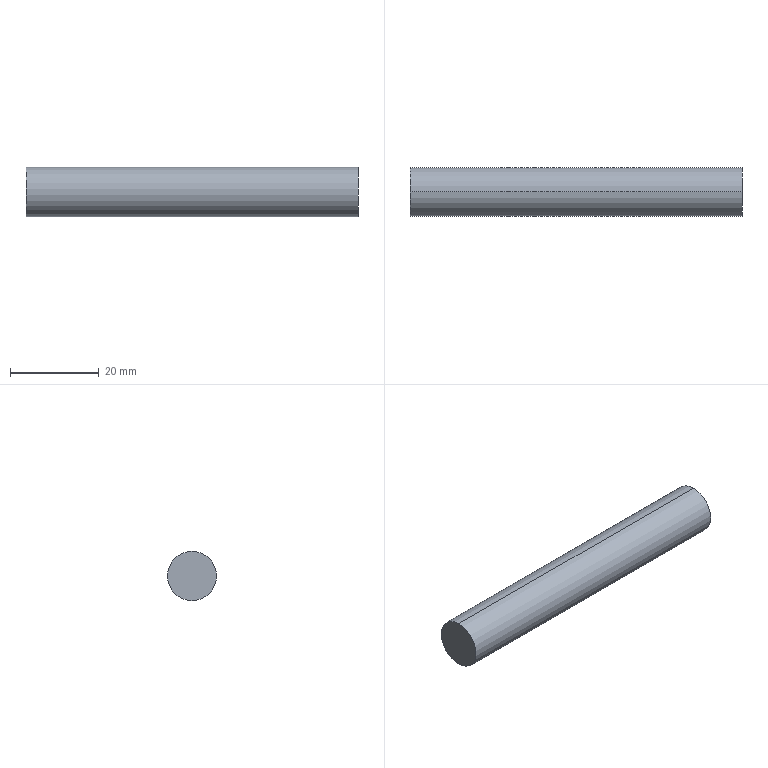Part | STEP file | 4-20.sldasm-Part-347 | 1 solid | 4 faces | box 75 x 11.11 x 11.11 mm | volume 7271 mm3 | cylinder 2 | plane 2 | commonest cylinder face diameters 11.11 x2
STEP:
#1=CARTESIAN_POINT('',(50.,-55.,84.445));
#2=VERTEX_POINT('',#1);
#3=CARTESIAN_POINT('',(50.,-55.,95.555));
#4=VERTEX_POINT('',#3);
#5=CARTESIAN_POINT('',(50.,-55.,90.));
#6=DIRECTION('',(-1.,0.,0.));
#7=DIRECTION('',(0.,0.,1.));
#8=AXIS2_PLACEMENT_3D('',#5,#6,#7);
#9=CIRCLE('',#8,5.555);
#10=EDGE_CURVE('',#2,#4,#9,.T.);
#11=ORIENTED_EDGE('',*,*,#10,.F.);
#12=CARTESIAN_POINT('',(125.,-55.,84.445));
#13=VERTEX_POINT('',#12);
#14=CARTESIAN_POINT('',(50.,-55.,84.445));
#15=DIRECTION('',(1.,0.,0.));
#16=VECTOR('',#15,1000.);
#17=LINE('',#14,#16);
#18=EDGE_CURVE('',#2,#13,#17,.T.);
#19=ORIENTED_EDGE('',*,*,#18,.T.);
#20=CARTESIAN_POINT('',(125.,-55.,95.555));
#21=VERTEX_POINT('',#20);
#22=CARTESIAN_POINT('',(125.,-55.,90.));
#23=DIRECTION('',(1.,0.,0.));
#24=DIRECTION('',(0.,0.,-1.));
#25=AXIS2_PLACEMENT_3D('',#22,#23,#24);
#26=CIRCLE('',#25,5.555);
#27=EDGE_CURVE('',#21,#13,#26,.T.);
#28=ORIENTED_EDGE('',*,*,#27,.F.);
#29=CARTESIAN_POINT('',(50.,-55.,95.555));
#30=DIRECTION('',(1.,0.,0.));
#31=VECTOR('',#30,1000.);
#32=LINE('',#29,#31);
#33=EDGE_CURVE('',#4,#21,#32,.T.);
#34=ORIENTED_EDGE('',*,*,#33,.F.);
#35=EDGE_LOOP('',(#11,#19,#28,#34));
#36=FACE_OUTER_BOUND('',#35,.T.);
#37=CARTESIAN_POINT('',(50.,-55.,90.));
#38=DIRECTION('',(1.,0.,0.));
#39=DIRECTION('',(0.,0.,1.));
#40=AXIS2_PLACEMENT_3D('',#37,#38,#39);
#41=CYLINDRICAL_SURFACE('',#40,5.555);
#42=ADVANCED_FACE('',(#36),#41,.T.);
#43=ORIENTED_EDGE('',*,*,#18,.F.);
#44=CARTESIAN_POINT('',(50.,-55.,90.));
#45=DIRECTION('',(-1.,0.,0.));
#46=DIRECTION('',(0.,0.,1.));
#47=AXIS2_PLACEMENT_3D('',#44,#45,#46);
#48=CIRCLE('',#47,5.555);
#49=EDGE_CURVE('',#4,#2,#48,.T.);
#50=ORIENTED_EDGE('',*,*,#49,.F.);
#51=ORIENTED_EDGE('',*,*,#33,.T.);
#52=CARTESIAN_POINT('',(125.,-55.,90.));
#53=DIRECTION('',(1.,0.,0.));
#54=DIRECTION('',(0.,0.,-1.));
#55=AXIS2_PLACEMENT_3D('',#52,#53,#54);
#56=CIRCLE('',#55,5.555);
#57=EDGE_CURVE('',#13,#21,#56,.T.);
#58=ORIENTED_EDGE('',*,*,#57,.F.);
#59=EDGE_LOOP('',(#43,#50,#51,#58));
#60=FACE_OUTER_BOUND('',#59,.T.);
#61=CARTESIAN_POINT('',(50.,-55.,90.));
#62=DIRECTION('',(1.,0.,0.));
#63=DIRECTION('',(0.,0.,1.));
#64=AXIS2_PLACEMENT_3D('',#61,#62,#63);
#65=CYLINDRICAL_SURFACE('',#64,5.555);
#66=ADVANCED_FACE('',(#60),#65,.T.);
#67=ORIENTED_EDGE('',*,*,#49,.T.);
#68=ORIENTED_EDGE('',*,*,#10,.T.);
#69=EDGE_LOOP('',(#67,#68));
#70=FACE_OUTER_BOUND('',#69,.T.);
#71=CARTESIAN_POINT('',(50.,-55.,90.));
#72=DIRECTION('',(-1.,0.,0.));
#73=DIRECTION('',(0.,0.,-1.));
#74=AXIS2_PLACEMENT_3D('',#71,#72,#73);
#75=PLANE('',#74);
#76=ADVANCED_FACE('',(#70),#75,.T.);
#77=ORIENTED_EDGE('',*,*,#27,.T.);
#78=ORIENTED_EDGE('',*,*,#57,.T.);
#79=EDGE_LOOP('',(#77,#78));
#80=FACE_OUTER_BOUND('',#79,.T.);
#81=CARTESIAN_POINT('',(125.,315.,290.));
#82=DIRECTION('',(1.,0.,0.));
#83=DIRECTION('',(0.,0.,-1.));
#84=AXIS2_PLACEMENT_3D('',#81,#82,#83);
#85=PLANE('',#84);
#86=ADVANCED_FACE('',(#80),#85,.T.);
#87=CLOSED_SHELL('',(#42,#66,#76,#86));
#88=MANIFOLD_SOLID_BREP('',#87);
#89=CARTESIAN_POINT('',(0.,0.,0.));
#90=DIRECTION('',(0.,0.,1.));
#91=DIRECTION('',(1.,0.,0.));
#92=AXIS2_PLACEMENT_3D('',#89,#90,#91);
#93=(LENGTH_UNIT()NAMED_UNIT(*)SI_UNIT(.MILLI.,.METRE.));
#94=UNCERTAINTY_MEASURE_WITH_UNIT(LENGTH_MEASURE(0.00001),#93,'','');
#95=(NAMED_UNIT(*)PLANE_ANGLE_UNIT()SI_UNIT($,.RADIAN.));
#96=(NAMED_UNIT(*)SI_UNIT($,.STERADIAN.)SOLID_ANGLE_UNIT());
#97=(GEOMETRIC_REPRESENTATION_CONTEXT(3)GLOBAL_UNCERTAINTY_ASSIGNED_CONTEXT((#94))GLOBAL_UNIT_ASSIGNED_CONTEXT((#93,#95,#96))REPRESENTATION_CONTEXT('',''));
#98=ADVANCED_BREP_SHAPE_REPRESENTATION('',(#88,#92),#97);